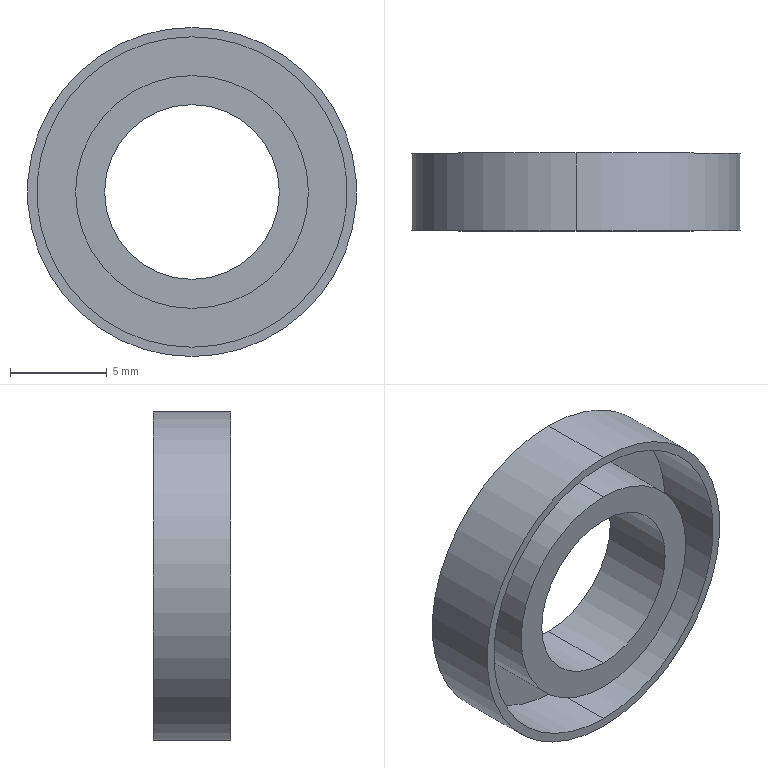Part | SolidWorks | features BaseBody 1 | 1 solid | 12 faces | box 16.96 x 4 x 16.96 mm | volume 341.308 mm3 | cylinder 8 | plane 4 | commonest cylinder face diameters 9 x2 12 x2 16 x2 16.96 x2
STEP:
#1=CARTESIAN_POINT('',(0.,-8.5,8.48));
#2=VERTEX_POINT('',#1);
#3=CARTESIAN_POINT('',(0.,-8.5,-8.48));
#4=VERTEX_POINT('',#3);
#5=CARTESIAN_POINT('',(0.,-8.5,0.));
#6=DIRECTION('',(0.,1.,0.));
#7=DIRECTION('',(0.,0.,1.));
#8=AXIS2_PLACEMENT_3D('',#5,#6,#7);
#9=CIRCLE('',#8,8.48);
#10=EDGE_CURVE('',#2,#4,#9,.T.);
#11=ORIENTED_EDGE('',*,*,#10,.T.);
#12=CARTESIAN_POINT('',(0.,-4.5,-8.48));
#13=VERTEX_POINT('',#12);
#14=CARTESIAN_POINT('',(0.,-6.5,-8.48));
#15=DIRECTION('',(0.,1.,0.));
#16=VECTOR('',#15,1000.);
#17=LINE('',#14,#16);
#18=EDGE_CURVE('',#4,#13,#17,.T.);
#19=ORIENTED_EDGE('',*,*,#18,.T.);
#20=CARTESIAN_POINT('',(0.,-4.5,8.48));
#21=VERTEX_POINT('',#20);
#22=CARTESIAN_POINT('',(0.,-4.5,0.));
#23=DIRECTION('',(0.,1.,0.));
#24=DIRECTION('',(0.,0.,1.));
#25=AXIS2_PLACEMENT_3D('',#22,#23,#24);
#26=CIRCLE('',#25,8.48);
#27=EDGE_CURVE('',#21,#13,#26,.T.);
#28=ORIENTED_EDGE('',*,*,#27,.F.);
#29=CARTESIAN_POINT('',(0.,-6.5,8.48));
#30=DIRECTION('',(0.,1.,0.));
#31=VECTOR('',#30,1000.);
#32=LINE('',#29,#31);
#33=EDGE_CURVE('',#2,#21,#32,.T.);
#34=ORIENTED_EDGE('',*,*,#33,.F.);
#35=EDGE_LOOP('',(#11,#19,#28,#34));
#36=FACE_OUTER_BOUND('',#35,.T.);
#37=CARTESIAN_POINT('',(0.,-6.5,0.));
#38=DIRECTION('',(0.,1.,0.));
#39=DIRECTION('',(0.,0.,1.));
#40=AXIS2_PLACEMENT_3D('',#37,#38,#39);
#41=CYLINDRICAL_SURFACE('',#40,8.48);
#42=ADVANCED_FACE('',(#36),#41,.T.);
#43=CARTESIAN_POINT('',(0.,-8.5,-4.5));
#44=VERTEX_POINT('',#43);
#45=CARTESIAN_POINT('',(0.,-8.5,4.5));
#46=VERTEX_POINT('',#45);
#47=CARTESIAN_POINT('',(0.,-8.5,0.));
#48=DIRECTION('',(0.,1.,0.));
#49=DIRECTION('',(0.,0.,1.));
#50=AXIS2_PLACEMENT_3D('',#47,#48,#49);
#51=CIRCLE('',#50,4.5);
#52=EDGE_CURVE('',#44,#46,#51,.T.);
#53=ORIENTED_EDGE('',*,*,#52,.F.);
#54=CARTESIAN_POINT('',(0.,-4.5,-4.5));
#55=VERTEX_POINT('',#54);
#56=CARTESIAN_POINT('',(0.,-6.5,-4.5));
#57=DIRECTION('',(0.,1.,0.));
#58=VECTOR('',#57,1000.);
#59=LINE('',#56,#58);
#60=EDGE_CURVE('',#44,#55,#59,.T.);
#61=ORIENTED_EDGE('',*,*,#60,.T.);
#62=CARTESIAN_POINT('',(0.,-4.5,4.5));
#63=VERTEX_POINT('',#62);
#64=CARTESIAN_POINT('',(0.,-4.5,0.));
#65=DIRECTION('',(0.,-1.,0.));
#66=DIRECTION('',(0.,0.,1.));
#67=AXIS2_PLACEMENT_3D('',#64,#65,#66);
#68=CIRCLE('',#67,4.5);
#69=EDGE_CURVE('',#63,#55,#68,.T.);
#70=ORIENTED_EDGE('',*,*,#69,.F.);
#71=CARTESIAN_POINT('',(0.,-6.5,4.5));
#72=DIRECTION('',(0.,1.,0.));
#73=VECTOR('',#72,1000.);
#74=LINE('',#71,#73);
#75=EDGE_CURVE('',#46,#63,#74,.T.);
#76=ORIENTED_EDGE('',*,*,#75,.F.);
#77=EDGE_LOOP('',(#53,#61,#70,#76));
#78=FACE_OUTER_BOUND('',#77,.T.);
#79=CARTESIAN_POINT('',(0.,-6.5,0.));
#80=DIRECTION('',(0.,1.,0.));
#81=DIRECTION('',(0.,0.,1.));
#82=AXIS2_PLACEMENT_3D('',#79,#80,#81);
#83=CYLINDRICAL_SURFACE('',#82,4.5);
#84=ADVANCED_FACE('',(#78),#83,.F.);
#85=CARTESIAN_POINT('',(0.,-8.5,-8.));
#86=VERTEX_POINT('',#85);
#87=CARTESIAN_POINT('',(0.,-8.5,8.));
#88=VERTEX_POINT('',#87);
#89=CARTESIAN_POINT('',(0.,-8.5,0.));
#90=DIRECTION('',(0.,1.,0.));
#91=DIRECTION('',(0.,0.,1.));
#92=AXIS2_PLACEMENT_3D('',#89,#90,#91);
#93=CIRCLE('',#92,8.);
#94=EDGE_CURVE('',#86,#88,#93,.T.);
#95=ORIENTED_EDGE('',*,*,#94,.F.);
#96=CARTESIAN_POINT('',(0.,-5.,-8.));
#97=VERTEX_POINT('',#96);
#98=CARTESIAN_POINT('',(0.,-6.75,-8.));
#99=DIRECTION('',(0.,1.,0.));
#100=VECTOR('',#99,1000.);
#101=LINE('',#98,#100);
#102=EDGE_CURVE('',#86,#97,#101,.T.);
#103=ORIENTED_EDGE('',*,*,#102,.T.);
#104=CARTESIAN_POINT('',(0.,-5.,8.));
#105=VERTEX_POINT('',#104);
#106=CARTESIAN_POINT('',(0.,-5.,0.));
#107=DIRECTION('',(0.,-1.,0.));
#108=DIRECTION('',(0.,0.,1.));
#109=AXIS2_PLACEMENT_3D('',#106,#107,#108);
#110=CIRCLE('',#109,8.);
#111=EDGE_CURVE('',#105,#97,#110,.T.);
#112=ORIENTED_EDGE('',*,*,#111,.F.);
#113=CARTESIAN_POINT('',(0.,-6.75,8.));
#114=DIRECTION('',(0.,1.,0.));
#115=VECTOR('',#114,1000.);
#116=LINE('',#113,#115);
#117=EDGE_CURVE('',#88,#105,#116,.T.);
#118=ORIENTED_EDGE('',*,*,#117,.F.);
#119=EDGE_LOOP('',(#95,#103,#112,#118));
#120=FACE_OUTER_BOUND('',#119,.T.);
#121=CARTESIAN_POINT('',(0.,-6.75,0.));
#122=DIRECTION('',(0.,1.,0.));
#123=DIRECTION('',(0.,0.,1.));
#124=AXIS2_PLACEMENT_3D('',#121,#122,#123);
#125=CYLINDRICAL_SURFACE('',#124,8.);
#126=ADVANCED_FACE('',(#120),#125,.F.);
#127=CARTESIAN_POINT('',(0.,-8.5,-6.));
#128=VERTEX_POINT('',#127);
#129=CARTESIAN_POINT('',(0.,-8.5,6.));
#130=VERTEX_POINT('',#129);
#131=CARTESIAN_POINT('',(0.,-8.5,0.));
#132=DIRECTION('',(0.,-1.,0.));
#133=DIRECTION('',(0.,0.,1.));
#134=AXIS2_PLACEMENT_3D('',#131,#132,#133);
#135=CIRCLE('',#134,6.);
#136=EDGE_CURVE('',#128,#130,#135,.T.);
#137=ORIENTED_EDGE('',*,*,#136,.F.);
#138=CARTESIAN_POINT('',(0.,-5.,-6.));
#139=VERTEX_POINT('',#138);
#140=CARTESIAN_POINT('',(0.,-6.5,-6.));
#141=DIRECTION('',(0.,1.,0.));
#142=VECTOR('',#141,1000.);
#143=LINE('',#140,#142);
#144=EDGE_CURVE('',#128,#139,#143,.T.);
#145=ORIENTED_EDGE('',*,*,#144,.T.);
#146=CARTESIAN_POINT('',(0.,-5.,6.));
#147=VERTEX_POINT('',#146);
#148=CARTESIAN_POINT('',(0.,-5.,0.));
#149=DIRECTION('',(0.,-1.,0.));
#150=DIRECTION('',(0.,0.,1.));
#151=AXIS2_PLACEMENT_3D('',#148,#149,#150);
#152=CIRCLE('',#151,6.);
#153=EDGE_CURVE('',#139,#147,#152,.T.);
#154=ORIENTED_EDGE('',*,*,#153,.T.);
#155=CARTESIAN_POINT('',(0.,-6.5,6.));
#156=DIRECTION('',(0.,1.,0.));
#157=VECTOR('',#156,1000.);
#158=LINE('',#155,#157);
#159=EDGE_CURVE('',#130,#147,#158,.T.);
#160=ORIENTED_EDGE('',*,*,#159,.F.);
#161=EDGE_LOOP('',(#137,#145,#154,#160));
#162=FACE_OUTER_BOUND('',#161,.T.);
#163=CARTESIAN_POINT('',(0.,-6.5,0.));
#164=DIRECTION('',(0.,1.,0.));
#165=DIRECTION('',(0.,0.,1.));
#166=AXIS2_PLACEMENT_3D('',#163,#164,#165);
#167=CYLINDRICAL_SURFACE('',#166,6.);
#168=ADVANCED_FACE('',(#162),#167,.T.);
#169=ORIENTED_EDGE('',*,*,#27,.T.);
#170=CARTESIAN_POINT('',(0.,-4.5,0.));
#171=DIRECTION('',(0.,1.,0.));
#172=DIRECTION('',(0.,0.,1.));
#173=AXIS2_PLACEMENT_3D('',#170,#171,#172);
#174=CIRCLE('',#173,8.48);
#175=EDGE_CURVE('',#13,#21,#174,.T.);
#176=ORIENTED_EDGE('',*,*,#175,.T.);
#177=EDGE_LOOP('',(#169,#176));
#178=FACE_OUTER_BOUND('',#177,.T.);
#179=ORIENTED_EDGE('',*,*,#69,.T.);
#180=CARTESIAN_POINT('',(0.,-4.5,0.));
#181=DIRECTION('',(0.,-1.,0.));
#182=DIRECTION('',(0.,0.,1.));
#183=AXIS2_PLACEMENT_3D('',#180,#181,#182);
#184=CIRCLE('',#183,4.5);
#185=EDGE_CURVE('',#55,#63,#184,.T.);
#186=ORIENTED_EDGE('',*,*,#185,.T.);
#187=EDGE_LOOP('',(#179,#186));
#188=FACE_BOUND('',#187,.T.);
#189=CARTESIAN_POINT('',(0.,-4.5,0.));
#190=DIRECTION('',(0.,1.,0.));
#191=DIRECTION('',(0.,0.,1.));
#192=AXIS2_PLACEMENT_3D('',#189,#190,#191);
#193=PLANE('',#192);
#194=ADVANCED_FACE('',(#178,#188),#193,.T.);
#195=ORIENTED_EDGE('',*,*,#18,.F.);
#196=CARTESIAN_POINT('',(0.,-8.5,0.));
#197=DIRECTION('',(0.,1.,0.));
#198=DIRECTION('',(0.,0.,1.));
#199=AXIS2_PLACEMENT_3D('',#196,#197,#198);
#200=CIRCLE('',#199,8.48);
#201=EDGE_CURVE('',#4,#2,#200,.T.);
#202=ORIENTED_EDGE('',*,*,#201,.T.);
#203=ORIENTED_EDGE('',*,*,#33,.T.);
#204=ORIENTED_EDGE('',*,*,#175,.F.);
#205=EDGE_LOOP('',(#195,#202,#203,#204));
#206=FACE_OUTER_BOUND('',#205,.T.);
#207=CARTESIAN_POINT('',(0.,-6.5,0.));
#208=DIRECTION('',(0.,1.,0.));
#209=DIRECTION('',(0.,0.,1.));
#210=AXIS2_PLACEMENT_3D('',#207,#208,#209);
#211=CYLINDRICAL_SURFACE('',#210,8.48);
#212=ADVANCED_FACE('',(#206),#211,.T.);
#213=ORIENTED_EDGE('',*,*,#60,.F.);
#214=CARTESIAN_POINT('',(0.,-8.5,0.));
#215=DIRECTION('',(0.,1.,0.));
#216=DIRECTION('',(0.,0.,1.));
#217=AXIS2_PLACEMENT_3D('',#214,#215,#216);
#218=CIRCLE('',#217,4.5);
#219=EDGE_CURVE('',#46,#44,#218,.T.);
#220=ORIENTED_EDGE('',*,*,#219,.F.);
#221=ORIENTED_EDGE('',*,*,#75,.T.);
#222=ORIENTED_EDGE('',*,*,#185,.F.);
#223=EDGE_LOOP('',(#213,#220,#221,#222));
#224=FACE_OUTER_BOUND('',#223,.T.);
#225=CARTESIAN_POINT('',(0.,-6.5,0.));
#226=DIRECTION('',(0.,1.,0.));
#227=DIRECTION('',(0.,0.,1.));
#228=AXIS2_PLACEMENT_3D('',#225,#226,#227);
#229=CYLINDRICAL_SURFACE('',#228,4.5);
#230=ADVANCED_FACE('',(#224),#229,.F.);
#231=ORIENTED_EDGE('',*,*,#10,.F.);
#232=ORIENTED_EDGE('',*,*,#201,.F.);
#233=EDGE_LOOP('',(#231,#232));
#234=FACE_OUTER_BOUND('',#233,.T.);
#235=CARTESIAN_POINT('',(0.,-8.5,0.));
#236=DIRECTION('',(0.,1.,0.));
#237=DIRECTION('',(0.,0.,1.));
#238=AXIS2_PLACEMENT_3D('',#235,#236,#237);
#239=CIRCLE('',#238,8.);
#240=EDGE_CURVE('',#88,#86,#239,.T.);
#241=ORIENTED_EDGE('',*,*,#240,.T.);
#242=ORIENTED_EDGE('',*,*,#94,.T.);
#243=EDGE_LOOP('',(#241,#242));
#244=FACE_BOUND('',#243,.T.);
#245=CARTESIAN_POINT('',(0.,-8.5,0.));
#246=DIRECTION('',(0.,-1.,0.));
#247=DIRECTION('',(0.,0.,-1.));
#248=AXIS2_PLACEMENT_3D('',#245,#246,#247);
#249=PLANE('',#248);
#250=ADVANCED_FACE('',(#234,#244),#249,.T.);
#251=CARTESIAN_POINT('',(0.,-8.5,0.));
#252=DIRECTION('',(0.,-1.,0.));
#253=DIRECTION('',(0.,0.,1.));
#254=AXIS2_PLACEMENT_3D('',#251,#252,#253);
#255=CIRCLE('',#254,6.);
#256=EDGE_CURVE('',#130,#128,#255,.T.);
#257=ORIENTED_EDGE('',*,*,#256,.T.);
#258=ORIENTED_EDGE('',*,*,#136,.T.);
#259=EDGE_LOOP('',(#257,#258));
#260=FACE_OUTER_BOUND('',#259,.T.);
#261=ORIENTED_EDGE('',*,*,#219,.T.);
#262=ORIENTED_EDGE('',*,*,#52,.T.);
#263=EDGE_LOOP('',(#261,#262));
#264=FACE_BOUND('',#263,.T.);
#265=CARTESIAN_POINT('',(0.,-8.5,0.));
#266=DIRECTION('',(0.,-1.,0.));
#267=DIRECTION('',(0.,0.,-1.));
#268=AXIS2_PLACEMENT_3D('',#265,#266,#267);
#269=PLANE('',#268);
#270=ADVANCED_FACE('',(#260,#264),#269,.T.);
#271=ORIENTED_EDGE('',*,*,#102,.F.);
#272=ORIENTED_EDGE('',*,*,#240,.F.);
#273=ORIENTED_EDGE('',*,*,#117,.T.);
#274=CARTESIAN_POINT('',(0.,-5.,0.));
#275=DIRECTION('',(0.,-1.,0.));
#276=DIRECTION('',(0.,0.,1.));
#277=AXIS2_PLACEMENT_3D('',#274,#275,#276);
#278=CIRCLE('',#277,8.);
#279=EDGE_CURVE('',#97,#105,#278,.T.);
#280=ORIENTED_EDGE('',*,*,#279,.F.);
#281=EDGE_LOOP('',(#271,#272,#273,#280));
#282=FACE_OUTER_BOUND('',#281,.T.);
#283=CARTESIAN_POINT('',(0.,-6.75,0.));
#284=DIRECTION('',(0.,1.,0.));
#285=DIRECTION('',(0.,0.,1.));
#286=AXIS2_PLACEMENT_3D('',#283,#284,#285);
#287=CYLINDRICAL_SURFACE('',#286,8.);
#288=ADVANCED_FACE('',(#282),#287,.F.);
#289=ORIENTED_EDGE('',*,*,#144,.F.);
#290=ORIENTED_EDGE('',*,*,#256,.F.);
#291=ORIENTED_EDGE('',*,*,#159,.T.);
#292=CARTESIAN_POINT('',(0.,-5.,0.));
#293=DIRECTION('',(0.,-1.,0.));
#294=DIRECTION('',(0.,0.,1.));
#295=AXIS2_PLACEMENT_3D('',#292,#293,#294);
#296=CIRCLE('',#295,6.);
#297=EDGE_CURVE('',#147,#139,#296,.T.);
#298=ORIENTED_EDGE('',*,*,#297,.T.);
#299=EDGE_LOOP('',(#289,#290,#291,#298));
#300=FACE_OUTER_BOUND('',#299,.T.);
#301=CARTESIAN_POINT('',(0.,-6.5,0.));
#302=DIRECTION('',(0.,1.,0.));
#303=DIRECTION('',(0.,0.,1.));
#304=AXIS2_PLACEMENT_3D('',#301,#302,#303);
#305=CYLINDRICAL_SURFACE('',#304,6.);
#306=ADVANCED_FACE('',(#300),#305,.T.);
#307=ORIENTED_EDGE('',*,*,#111,.T.);
#308=ORIENTED_EDGE('',*,*,#279,.T.);
#309=EDGE_LOOP('',(#307,#308));
#310=FACE_OUTER_BOUND('',#309,.T.);
#311=ORIENTED_EDGE('',*,*,#297,.F.);
#312=ORIENTED_EDGE('',*,*,#153,.F.);
#313=EDGE_LOOP('',(#311,#312));
#314=FACE_BOUND('',#313,.T.);
#315=CARTESIAN_POINT('',(0.,-5.,0.));
#316=DIRECTION('',(0.,1.,0.));
#317=DIRECTION('',(0.,0.,1.));
#318=AXIS2_PLACEMENT_3D('',#315,#316,#317);
#319=PLANE('',#318);
#320=ADVANCED_FACE('',(#310,#314),#319,.F.);
#321=CLOSED_SHELL('',(#42,#84,#126,#168,#194,#212,#230,#250,#270,#288,#306,#320));
#322=MANIFOLD_SOLID_BREP('',#321);
#323=CARTESIAN_POINT('',(0.,0.,0.));
#324=DIRECTION('',(0.,0.,1.));
#325=DIRECTION('',(1.,0.,0.));
#326=AXIS2_PLACEMENT_3D('',#323,#324,#325);
#327=(LENGTH_UNIT()NAMED_UNIT(*)SI_UNIT(.MILLI.,.METRE.));
#328=UNCERTAINTY_MEASURE_WITH_UNIT(LENGTH_MEASURE(0.00001),#327,'','');
#329=(NAMED_UNIT(*)PLANE_ANGLE_UNIT()SI_UNIT($,.RADIAN.));
#330=(NAMED_UNIT(*)SI_UNIT($,.STERADIAN.)SOLID_ANGLE_UNIT());
#331=(GEOMETRIC_REPRESENTATION_CONTEXT(3)GLOBAL_UNCERTAINTY_ASSIGNED_CONTEXT((#328))GLOBAL_UNIT_ASSIGNED_CONTEXT((#327,#329,#330))REPRESENTATION_CONTEXT('',''));
#332=ADVANCED_BREP_SHAPE_REPRESENTATION('',(#322,#326),#331);